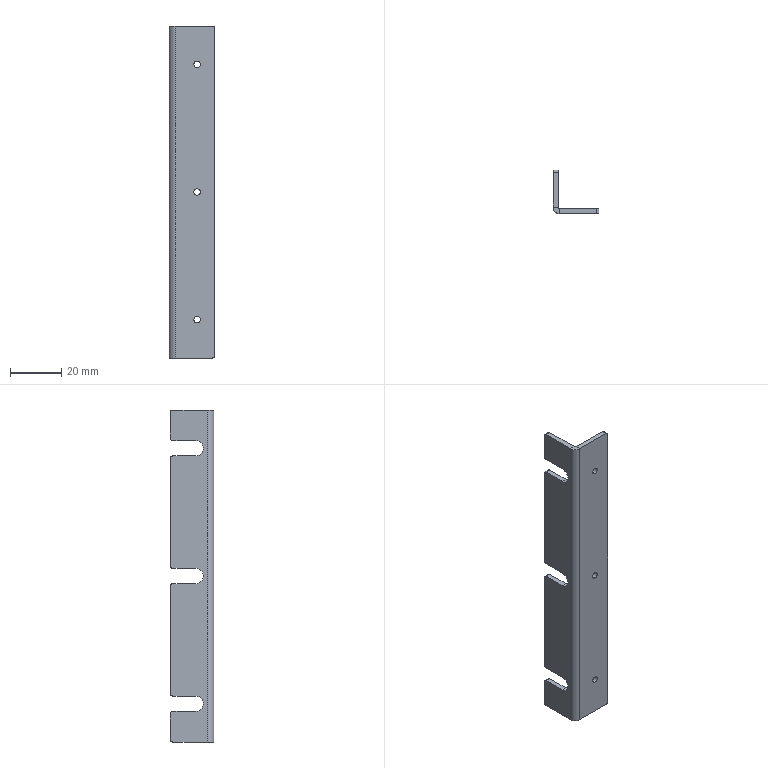Part | STEP file | 1 solid | 42 faces | box 18 x 17 x 130 mm | volume 7934 mm3 | cylinder 21 | plane 21 | commonest cylinder face diameters 2 x10 2.5 x6 6 x3 1 x1 5 x1